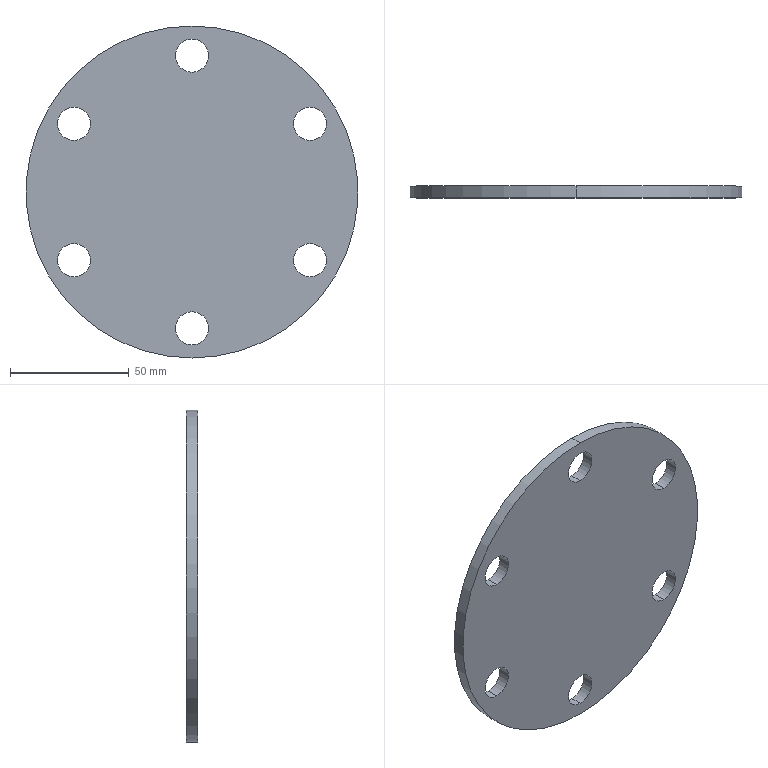Part | STEP file | OP10-030_plate | 1 solid | 16 faces | box 140 x 5 x 140 mm | volume 72351 mm3 | cylinder 14 | plane 2 | commonest cylinder face diameters 14 x12 140 x2
STEP:
#1=CARTESIAN_POINT('',(0.,0.,0.));
#2=DIRECTION('',(0.,0.,1.));
#3=DIRECTION('',(1.,0.,0.));
#4=AXIS2_PLACEMENT_3D('',#1,#2,#3);
#5=CARTESIAN_POINT('',(-49.796,0.,-21.75));
#6=VERTEX_POINT('',#5);
#7=CARTESIAN_POINT('',(-49.796,5.,-21.75));
#8=VERTEX_POINT('',#7);
#9=CARTESIAN_POINT('',(-49.796,0.,-21.75));
#10=DIRECTION('',(0.,1.,0.));
#11=VECTOR('',#10,1.);
#12=LINE('',#9,#11);
#13=CARTESIAN_POINT('',(-49.796,0.,-28.75));
#14=DIRECTION('',(0.,1.,0.));
#15=DIRECTION('',(0.,0.,1.));
#16=AXIS2_PLACEMENT_3D('',#13,#14,#15);
#17=CYLINDRICAL_SURFACE('',#16,7.);
#18=CARTESIAN_POINT('',(6.283,0.));
#19=DIRECTION('',(0.,1.));
#20=VECTOR('',#19,1.);
#21=LINE('',#18,#20);
#22=(GEOMETRIC_REPRESENTATION_CONTEXT(2)PARAMETRIC_REPRESENTATION_CONTEXT()REPRESENTATION_CONTEXT('',''));
#23=DEFINITIONAL_REPRESENTATION('',(#21),#22);
#24=PCURVE('',#17,#23);
#25=CARTESIAN_POINT('',(-49.796,0.,-28.75));
#26=DIRECTION('',(0.,1.,0.));
#27=DIRECTION('',(0.,0.,1.));
#28=AXIS2_PLACEMENT_3D('',#25,#26,#27);
#29=CYLINDRICAL_SURFACE('',#28,7.);
#30=CARTESIAN_POINT('',(0.,0.));
#31=DIRECTION('',(0.,1.));
#32=VECTOR('',#31,1.);
#33=LINE('',#30,#32);
#34=(GEOMETRIC_REPRESENTATION_CONTEXT(2)PARAMETRIC_REPRESENTATION_CONTEXT()REPRESENTATION_CONTEXT('',''));
#35=DEFINITIONAL_REPRESENTATION('',(#33),#34);
#36=PCURVE('',#29,#35);
#37=SURFACE_CURVE('',#12,(#24,#36),.PCURVE_S1.);
#38=EDGE_CURVE('',#6,#8,#37,.T.);
#39=ORIENTED_EDGE('',*,*,#38,.T.);
#40=CARTESIAN_POINT('',(-49.796,5.,-35.75));
#41=VERTEX_POINT('',#40);
#42=CARTESIAN_POINT('',(-49.796,5.,-28.75));
#43=DIRECTION('',(0.,1.,0.));
#44=DIRECTION('',(0.866,0.,0.5));
#45=AXIS2_PLACEMENT_3D('',#42,#43,#44);
#46=CIRCLE('',#45,7.);
#47=CARTESIAN_POINT('',(1.047,5.));
#48=DIRECTION('',(1.,0.));
#49=VECTOR('',#48,1.);
#50=LINE('',#47,#49);
#51=(GEOMETRIC_REPRESENTATION_CONTEXT(2)PARAMETRIC_REPRESENTATION_CONTEXT()REPRESENTATION_CONTEXT('',''));
#52=DEFINITIONAL_REPRESENTATION('',(#50),#51);
#53=PCURVE('',#17,#52);
#54=CARTESIAN_POINT('',(0.,5.,0.));
#55=DIRECTION('',(0.,1.,0.));
#56=DIRECTION('',(0.,0.,1.));
#57=AXIS2_PLACEMENT_3D('',#54,#55,#56);
#58=PLANE('',#57);
#59=CARTESIAN_POINT('',(-28.75,-49.796));
#60=DIRECTION('',(0.5,0.866));
#61=AXIS2_PLACEMENT_2D('',#59,#60);
#62=CIRCLE('',#61,7.);
#63=(GEOMETRIC_REPRESENTATION_CONTEXT(2)PARAMETRIC_REPRESENTATION_CONTEXT()REPRESENTATION_CONTEXT('',''));
#64=DEFINITIONAL_REPRESENTATION('',(#62),#63);
#65=PCURVE('',#58,#64);
#66=SURFACE_CURVE('',#46,(#53,#65),.PCURVE_S1.);
#67=EDGE_CURVE('',#41,#8,#66,.T.);
#68=ORIENTED_EDGE('',*,*,#67,.F.);
#69=CARTESIAN_POINT('',(-49.796,0.,-35.75));
#70=VERTEX_POINT('',#69);
#71=CARTESIAN_POINT('',(-49.796,0.,-35.75));
#72=DIRECTION('',(0.,1.,0.));
#73=VECTOR('',#72,1.);
#74=LINE('',#71,#73);
#75=CARTESIAN_POINT('',(3.142,0.));
#76=DIRECTION('',(0.,1.));
#77=VECTOR('',#76,1.);
#78=LINE('',#75,#77);
#79=(GEOMETRIC_REPRESENTATION_CONTEXT(2)PARAMETRIC_REPRESENTATION_CONTEXT()REPRESENTATION_CONTEXT('',''));
#80=DEFINITIONAL_REPRESENTATION('',(#78),#79);
#81=PCURVE('',#17,#80);
#82=CARTESIAN_POINT('',(3.142,0.));
#83=DIRECTION('',(0.,1.));
#84=VECTOR('',#83,1.);
#85=LINE('',#82,#84);
#86=(GEOMETRIC_REPRESENTATION_CONTEXT(2)PARAMETRIC_REPRESENTATION_CONTEXT()REPRESENTATION_CONTEXT('',''));
#87=DEFINITIONAL_REPRESENTATION('',(#85),#86);
#88=PCURVE('',#29,#87);
#89=SURFACE_CURVE('',#74,(#81,#88),.PCURVE_S1.);
#90=EDGE_CURVE('',#70,#41,#89,.T.);
#91=ORIENTED_EDGE('',*,*,#90,.F.);
#92=CARTESIAN_POINT('',(-49.796,0.,-28.75));
#93=DIRECTION('',(0.,1.,0.));
#94=DIRECTION('',(0.866,0.,0.5));
#95=AXIS2_PLACEMENT_3D('',#92,#93,#94);
#96=CIRCLE('',#95,7.);
#97=CARTESIAN_POINT('',(1.047,0.));
#98=DIRECTION('',(1.,0.));
#99=VECTOR('',#98,1.);
#100=LINE('',#97,#99);
#101=(GEOMETRIC_REPRESENTATION_CONTEXT(2)PARAMETRIC_REPRESENTATION_CONTEXT()REPRESENTATION_CONTEXT('',''));
#102=DEFINITIONAL_REPRESENTATION('',(#100),#101);
#103=PCURVE('',#17,#102);
#104=CARTESIAN_POINT('',(0.,0.,0.));
#105=DIRECTION('',(0.,1.,0.));
#106=DIRECTION('',(0.,0.,1.));
#107=AXIS2_PLACEMENT_3D('',#104,#105,#106);
#108=PLANE('',#107);
#109=CARTESIAN_POINT('',(-28.75,-49.796));
#110=DIRECTION('',(0.5,0.866));
#111=AXIS2_PLACEMENT_2D('',#109,#110);
#112=CIRCLE('',#111,7.);
#113=(GEOMETRIC_REPRESENTATION_CONTEXT(2)PARAMETRIC_REPRESENTATION_CONTEXT()REPRESENTATION_CONTEXT('',''));
#114=DEFINITIONAL_REPRESENTATION('',(#112),#113);
#115=PCURVE('',#108,#114);
#116=SURFACE_CURVE('',#96,(#103,#115),.PCURVE_S1.);
#117=EDGE_CURVE('',#70,#6,#116,.T.);
#118=ORIENTED_EDGE('',*,*,#117,.T.);
#119=EDGE_LOOP('',(#39,#68,#91,#118));
#120=FACE_BOUND('',#119,.F.);
#121=ADVANCED_FACE('',(#120),#17,.F.);
#122=CARTESIAN_POINT('',(-49.796,0.,35.75));
#123=VERTEX_POINT('',#122);
#124=CARTESIAN_POINT('',(-49.796,5.,35.75));
#125=VERTEX_POINT('',#124);
#126=CARTESIAN_POINT('',(-49.796,0.,35.75));
#127=DIRECTION('',(0.,1.,0.));
#128=VECTOR('',#127,1.);
#129=LINE('',#126,#128);
#130=CARTESIAN_POINT('',(-49.796,0.,28.75));
#131=DIRECTION('',(0.,1.,0.));
#132=DIRECTION('',(0.,0.,1.));
#133=AXIS2_PLACEMENT_3D('',#130,#131,#132);
#134=CYLINDRICAL_SURFACE('',#133,7.);
#135=CARTESIAN_POINT('',(6.283,0.));
#136=DIRECTION('',(0.,1.));
#137=VECTOR('',#136,1.);
#138=LINE('',#135,#137);
#139=(GEOMETRIC_REPRESENTATION_CONTEXT(2)PARAMETRIC_REPRESENTATION_CONTEXT()REPRESENTATION_CONTEXT('',''));
#140=DEFINITIONAL_REPRESENTATION('',(#138),#139);
#141=PCURVE('',#134,#140);
#142=CARTESIAN_POINT('',(-49.796,0.,28.75));
#143=DIRECTION('',(0.,1.,0.));
#144=DIRECTION('',(0.,0.,1.));
#145=AXIS2_PLACEMENT_3D('',#142,#143,#144);
#146=CYLINDRICAL_SURFACE('',#145,7.);
#147=CARTESIAN_POINT('',(0.,0.));
#148=DIRECTION('',(0.,1.));
#149=VECTOR('',#148,1.);
#150=LINE('',#147,#149);
#151=(GEOMETRIC_REPRESENTATION_CONTEXT(2)PARAMETRIC_REPRESENTATION_CONTEXT()REPRESENTATION_CONTEXT('',''));
#152=DEFINITIONAL_REPRESENTATION('',(#150),#151);
#153=PCURVE('',#146,#152);
#154=SURFACE_CURVE('',#129,(#141,#153),.PCURVE_S1.);
#155=EDGE_CURVE('',#123,#125,#154,.T.);
#156=ORIENTED_EDGE('',*,*,#155,.T.);
#157=CARTESIAN_POINT('',(-49.796,5.,21.75));
#158=VERTEX_POINT('',#157);
#159=CARTESIAN_POINT('',(-49.796,5.,28.75));
#160=DIRECTION('',(0.,1.,0.));
#161=DIRECTION('',(0.866,0.,-0.5));
#162=AXIS2_PLACEMENT_3D('',#159,#160,#161);
#163=CIRCLE('',#162,7.);
#164=CARTESIAN_POINT('',(2.094,5.));
#165=DIRECTION('',(1.,0.));
#166=VECTOR('',#165,1.);
#167=LINE('',#164,#166);
#168=(GEOMETRIC_REPRESENTATION_CONTEXT(2)PARAMETRIC_REPRESENTATION_CONTEXT()REPRESENTATION_CONTEXT('',''));
#169=DEFINITIONAL_REPRESENTATION('',(#167),#168);
#170=PCURVE('',#134,#169);
#171=CARTESIAN_POINT('',(28.75,-49.796));
#172=DIRECTION('',(-0.5,0.866));
#173=AXIS2_PLACEMENT_2D('',#171,#172);
#174=CIRCLE('',#173,7.);
#175=(GEOMETRIC_REPRESENTATION_CONTEXT(2)PARAMETRIC_REPRESENTATION_CONTEXT()REPRESENTATION_CONTEXT('',''));
#176=DEFINITIONAL_REPRESENTATION('',(#174),#175);
#177=PCURVE('',#58,#176);
#178=SURFACE_CURVE('',#163,(#170,#177),.PCURVE_S1.);
#179=EDGE_CURVE('',#158,#125,#178,.T.);
#180=ORIENTED_EDGE('',*,*,#179,.F.);
#181=CARTESIAN_POINT('',(-49.796,0.,21.75));
#182=VERTEX_POINT('',#181);
#183=CARTESIAN_POINT('',(-49.796,0.,21.75));
#184=DIRECTION('',(0.,1.,0.));
#185=VECTOR('',#184,1.);
#186=LINE('',#183,#185);
#187=CARTESIAN_POINT('',(3.142,0.));
#188=DIRECTION('',(0.,1.));
#189=VECTOR('',#188,1.);
#190=LINE('',#187,#189);
#191=(GEOMETRIC_REPRESENTATION_CONTEXT(2)PARAMETRIC_REPRESENTATION_CONTEXT()REPRESENTATION_CONTEXT('',''));
#192=DEFINITIONAL_REPRESENTATION('',(#190),#191);
#193=PCURVE('',#134,#192);
#194=CARTESIAN_POINT('',(3.142,0.));
#195=DIRECTION('',(0.,1.));
#196=VECTOR('',#195,1.);
#197=LINE('',#194,#196);
#198=(GEOMETRIC_REPRESENTATION_CONTEXT(2)PARAMETRIC_REPRESENTATION_CONTEXT()REPRESENTATION_CONTEXT('',''));
#199=DEFINITIONAL_REPRESENTATION('',(#197),#198);
#200=PCURVE('',#146,#199);
#201=SURFACE_CURVE('',#186,(#193,#200),.PCURVE_S1.);
#202=EDGE_CURVE('',#182,#158,#201,.T.);
#203=ORIENTED_EDGE('',*,*,#202,.F.);
#204=CARTESIAN_POINT('',(-49.796,0.,28.75));
#205=DIRECTION('',(0.,1.,0.));
#206=DIRECTION('',(0.866,0.,-0.5));
#207=AXIS2_PLACEMENT_3D('',#204,#205,#206);
#208=CIRCLE('',#207,7.);
#209=CARTESIAN_POINT('',(2.094,0.));
#210=DIRECTION('',(1.,0.));
#211=VECTOR('',#210,1.);
#212=LINE('',#209,#211);
#213=(GEOMETRIC_REPRESENTATION_CONTEXT(2)PARAMETRIC_REPRESENTATION_CONTEXT()REPRESENTATION_CONTEXT('',''));
#214=DEFINITIONAL_REPRESENTATION('',(#212),#213);
#215=PCURVE('',#134,#214);
#216=CARTESIAN_POINT('',(28.75,-49.796));
#217=DIRECTION('',(-0.5,0.866));
#218=AXIS2_PLACEMENT_2D('',#216,#217);
#219=CIRCLE('',#218,7.);
#220=(GEOMETRIC_REPRESENTATION_CONTEXT(2)PARAMETRIC_REPRESENTATION_CONTEXT()REPRESENTATION_CONTEXT('',''));
#221=DEFINITIONAL_REPRESENTATION('',(#219),#220);
#222=PCURVE('',#108,#221);
#223=SURFACE_CURVE('',#208,(#215,#222),.PCURVE_S1.);
#224=EDGE_CURVE('',#182,#123,#223,.T.);
#225=ORIENTED_EDGE('',*,*,#224,.T.);
#226=EDGE_LOOP('',(#156,#180,#203,#225));
#227=FACE_BOUND('',#226,.F.);
#228=ADVANCED_FACE('',(#227),#134,.F.);
#229=CARTESIAN_POINT('',(0.,0.,64.5));
#230=VERTEX_POINT('',#229);
#231=CARTESIAN_POINT('',(0.,5.,64.5));
#232=VERTEX_POINT('',#231);
#233=CARTESIAN_POINT('',(0.,0.,64.5));
#234=DIRECTION('',(0.,1.,0.));
#235=VECTOR('',#234,1.);
#236=LINE('',#233,#235);
#237=CARTESIAN_POINT('',(0.,0.,57.5));
#238=DIRECTION('',(0.,1.,0.));
#239=DIRECTION('',(0.,0.,1.));
#240=AXIS2_PLACEMENT_3D('',#237,#238,#239);
#241=CYLINDRICAL_SURFACE('',#240,7.);
#242=CARTESIAN_POINT('',(6.283,0.));
#243=DIRECTION('',(0.,1.));
#244=VECTOR('',#243,1.);
#245=LINE('',#242,#244);
#246=(GEOMETRIC_REPRESENTATION_CONTEXT(2)PARAMETRIC_REPRESENTATION_CONTEXT()REPRESENTATION_CONTEXT('',''));
#247=DEFINITIONAL_REPRESENTATION('',(#245),#246);
#248=PCURVE('',#241,#247);
#249=CARTESIAN_POINT('',(0.,0.,57.5));
#250=DIRECTION('',(0.,1.,0.));
#251=DIRECTION('',(0.,0.,1.));
#252=AXIS2_PLACEMENT_3D('',#249,#250,#251);
#253=CYLINDRICAL_SURFACE('',#252,7.);
#254=CARTESIAN_POINT('',(0.,0.));
#255=DIRECTION('',(0.,1.));
#256=VECTOR('',#255,1.);
#257=LINE('',#254,#256);
#258=(GEOMETRIC_REPRESENTATION_CONTEXT(2)PARAMETRIC_REPRESENTATION_CONTEXT()REPRESENTATION_CONTEXT('',''));
#259=DEFINITIONAL_REPRESENTATION('',(#257),#258);
#260=PCURVE('',#253,#259);
#261=SURFACE_CURVE('',#236,(#248,#260),.PCURVE_S1.);
#262=EDGE_CURVE('',#230,#232,#261,.T.);
#263=ORIENTED_EDGE('',*,*,#262,.T.);
#264=CARTESIAN_POINT('',(0.,5.,50.5));
#265=VERTEX_POINT('',#264);
#266=CARTESIAN_POINT('',(0.,5.,57.5));
#267=DIRECTION('',(0.,1.,0.));
#268=DIRECTION('',(0.,0.,-1.));
#269=AXIS2_PLACEMENT_3D('',#266,#267,#268);
#270=CIRCLE('',#269,7.);
#271=CARTESIAN_POINT('',(3.142,5.));
#272=DIRECTION('',(1.,0.));
#273=VECTOR('',#272,1.);
#274=LINE('',#271,#273);
#275=(GEOMETRIC_REPRESENTATION_CONTEXT(2)PARAMETRIC_REPRESENTATION_CONTEXT()REPRESENTATION_CONTEXT('',''));
#276=DEFINITIONAL_REPRESENTATION('',(#274),#275);
#277=PCURVE('',#241,#276);
#278=CARTESIAN_POINT('',(57.5,0.));
#279=DIRECTION('',(-1.,0.));
#280=AXIS2_PLACEMENT_2D('',#278,#279);
#281=CIRCLE('',#280,7.);
#282=(GEOMETRIC_REPRESENTATION_CONTEXT(2)PARAMETRIC_REPRESENTATION_CONTEXT()REPRESENTATION_CONTEXT('',''));
#283=DEFINITIONAL_REPRESENTATION('',(#281),#282);
#284=PCURVE('',#58,#283);
#285=SURFACE_CURVE('',#270,(#277,#284),.PCURVE_S1.);
#286=EDGE_CURVE('',#265,#232,#285,.T.);
#287=ORIENTED_EDGE('',*,*,#286,.F.);
#288=CARTESIAN_POINT('',(0.,0.,50.5));
#289=VERTEX_POINT('',#288);
#290=CARTESIAN_POINT('',(0.,0.,50.5));
#291=DIRECTION('',(0.,1.,0.));
#292=VECTOR('',#291,1.);
#293=LINE('',#290,#292);
#294=CARTESIAN_POINT('',(3.142,0.));
#295=DIRECTION('',(0.,1.));
#296=VECTOR('',#295,1.);
#297=LINE('',#294,#296);
#298=(GEOMETRIC_REPRESENTATION_CONTEXT(2)PARAMETRIC_REPRESENTATION_CONTEXT()REPRESENTATION_CONTEXT('',''));
#299=DEFINITIONAL_REPRESENTATION('',(#297),#298);
#300=PCURVE('',#241,#299);
#301=CARTESIAN_POINT('',(3.142,0.));
#302=DIRECTION('',(0.,1.));
#303=VECTOR('',#302,1.);
#304=LINE('',#301,#303);
#305=(GEOMETRIC_REPRESENTATION_CONTEXT(2)PARAMETRIC_REPRESENTATION_CONTEXT()REPRESENTATION_CONTEXT('',''));
#306=DEFINITIONAL_REPRESENTATION('',(#304),#305);
#307=PCURVE('',#253,#306);
#308=SURFACE_CURVE('',#293,(#300,#307),.PCURVE_S1.);
#309=EDGE_CURVE('',#289,#265,#308,.T.);
#310=ORIENTED_EDGE('',*,*,#309,.F.);
#311=CARTESIAN_POINT('',(0.,0.,57.5));
#312=DIRECTION('',(0.,1.,0.));
#313=DIRECTION('',(0.,0.,-1.));
#314=AXIS2_PLACEMENT_3D('',#311,#312,#313);
#315=CIRCLE('',#314,7.);
#316=CARTESIAN_POINT('',(3.142,0.));
#317=DIRECTION('',(1.,0.));
#318=VECTOR('',#317,1.);
#319=LINE('',#316,#318);
#320=(GEOMETRIC_REPRESENTATION_CONTEXT(2)PARAMETRIC_REPRESENTATION_CONTEXT()REPRESENTATION_CONTEXT('',''));
#321=DEFINITIONAL_REPRESENTATION('',(#319),#320);
#322=PCURVE('',#241,#321);
#323=CARTESIAN_POINT('',(57.5,0.));
#324=DIRECTION('',(-1.,0.));
#325=AXIS2_PLACEMENT_2D('',#323,#324);
#326=CIRCLE('',#325,7.);
#327=(GEOMETRIC_REPRESENTATION_CONTEXT(2)PARAMETRIC_REPRESENTATION_CONTEXT()REPRESENTATION_CONTEXT('',''));
#328=DEFINITIONAL_REPRESENTATION('',(#326),#327);
#329=PCURVE('',#108,#328);
#330=SURFACE_CURVE('',#315,(#322,#329),.PCURVE_S1.);
#331=EDGE_CURVE('',#289,#230,#330,.T.);
#332=ORIENTED_EDGE('',*,*,#331,.T.);
#333=EDGE_LOOP('',(#263,#287,#310,#332));
#334=FACE_BOUND('',#333,.F.);
#335=ADVANCED_FACE('',(#334),#241,.F.);
#336=CARTESIAN_POINT('',(49.796,0.,35.75));
#337=VERTEX_POINT('',#336);
#338=CARTESIAN_POINT('',(49.796,5.,35.75));
#339=VERTEX_POINT('',#338);
#340=CARTESIAN_POINT('',(49.796,0.,35.75));
#341=DIRECTION('',(0.,1.,0.));
#342=VECTOR('',#341,1.);
#343=LINE('',#340,#342);
#344=CARTESIAN_POINT('',(49.796,0.,28.75));
#345=DIRECTION('',(0.,1.,0.));
#346=DIRECTION('',(0.,0.,1.));
#347=AXIS2_PLACEMENT_3D('',#344,#345,#346);
#348=CYLINDRICAL_SURFACE('',#347,7.);
#349=CARTESIAN_POINT('',(6.283,0.));
#350=DIRECTION('',(0.,1.));
#351=VECTOR('',#350,1.);
#352=LINE('',#349,#351);
#353=(GEOMETRIC_REPRESENTATION_CONTEXT(2)PARAMETRIC_REPRESENTATION_CONTEXT()REPRESENTATION_CONTEXT('',''));
#354=DEFINITIONAL_REPRESENTATION('',(#352),#353);
#355=PCURVE('',#348,#354);
#356=CARTESIAN_POINT('',(49.796,0.,28.75));
#357=DIRECTION('',(0.,1.,0.));
#358=DIRECTION('',(0.,0.,1.));
#359=AXIS2_PLACEMENT_3D('',#356,#357,#358);
#360=CYLINDRICAL_SURFACE('',#359,7.);
#361=CARTESIAN_POINT('',(0.,0.));
#362=DIRECTION('',(0.,1.));
#363=VECTOR('',#362,1.);
#364=LINE('',#361,#363);
#365=(GEOMETRIC_REPRESENTATION_CONTEXT(2)PARAMETRIC_REPRESENTATION_CONTEXT()REPRESENTATION_CONTEXT('',''));
#366=DEFINITIONAL_REPRESENTATION('',(#364),#365);
#367=PCURVE('',#360,#366);
#368=SURFACE_CURVE('',#343,(#355,#367),.PCURVE_S1.);
#369=EDGE_CURVE('',#337,#339,#368,.T.);
#370=ORIENTED_EDGE('',*,*,#369,.T.);
#371=CARTESIAN_POINT('',(49.796,5.,21.75));
#372=VERTEX_POINT('',#371);
#373=CARTESIAN_POINT('',(49.796,5.,28.75));
#374=DIRECTION('',(0.,1.,0.));
#375=DIRECTION('',(-0.866,0.,-0.5));
#376=AXIS2_PLACEMENT_3D('',#373,#374,#375);
#377=CIRCLE('',#376,7.);
#378=CARTESIAN_POINT('',(-2.094,5.));
#379=DIRECTION('',(1.,0.));
#380=VECTOR('',#379,1.);
#381=LINE('',#378,#380);
#382=(GEOMETRIC_REPRESENTATION_CONTEXT(2)PARAMETRIC_REPRESENTATION_CONTEXT()REPRESENTATION_CONTEXT('',''));
#383=DEFINITIONAL_REPRESENTATION('',(#381),#382);
#384=PCURVE('',#348,#383);
#385=CARTESIAN_POINT('',(28.75,49.796));
#386=DIRECTION('',(-0.5,-0.866));
#387=AXIS2_PLACEMENT_2D('',#385,#386);
#388=CIRCLE('',#387,7.);
#389=(GEOMETRIC_REPRESENTATION_CONTEXT(2)PARAMETRIC_REPRESENTATION_CONTEXT()REPRESENTATION_CONTEXT('',''));
#390=DEFINITIONAL_REPRESENTATION('',(#388),#389);
#391=PCURVE('',#58,#390);
#392=SURFACE_CURVE('',#377,(#384,#391),.PCURVE_S1.);
#393=EDGE_CURVE('',#372,#339,#392,.T.);
#394=ORIENTED_EDGE('',*,*,#393,.F.);
#395=CARTESIAN_POINT('',(49.796,0.,21.75));
#396=VERTEX_POINT('',#395);
#397=CARTESIAN_POINT('',(49.796,0.,21.75));
#398=DIRECTION('',(0.,1.,0.));
#399=VECTOR('',#398,1.);
#400=LINE('',#397,#399);
#401=CARTESIAN_POINT('',(3.142,0.));
#402=DIRECTION('',(0.,1.));
#403=VECTOR('',#402,1.);
#404=LINE('',#401,#403);
#405=(GEOMETRIC_REPRESENTATION_CONTEXT(2)PARAMETRIC_REPRESENTATION_CONTEXT()REPRESENTATION_CONTEXT('',''));
#406=DEFINITIONAL_REPRESENTATION('',(#404),#405);
#407=PCURVE('',#348,#406);
#408=CARTESIAN_POINT('',(3.142,0.));
#409=DIRECTION('',(0.,1.));
#410=VECTOR('',#409,1.);
#411=LINE('',#408,#410);
#412=(GEOMETRIC_REPRESENTATION_CONTEXT(2)PARAMETRIC_REPRESENTATION_CONTEXT()REPRESENTATION_CONTEXT('',''));
#413=DEFINITIONAL_REPRESENTATION('',(#411),#412);
#414=PCURVE('',#360,#413);
#415=SURFACE_CURVE('',#400,(#407,#414),.PCURVE_S1.);
#416=EDGE_CURVE('',#396,#372,#415,.T.);
#417=ORIENTED_EDGE('',*,*,#416,.F.);
#418=CARTESIAN_POINT('',(49.796,0.,28.75));
#419=DIRECTION('',(0.,1.,0.));
#420=DIRECTION('',(-0.866,0.,-0.5));
#421=AXIS2_PLACEMENT_3D('',#418,#419,#420);
#422=CIRCLE('',#421,7.);
#423=CARTESIAN_POINT('',(-2.094,0.));
#424=DIRECTION('',(1.,0.));
#425=VECTOR('',#424,1.);
#426=LINE('',#423,#425);
#427=(GEOMETRIC_REPRESENTATION_CONTEXT(2)PARAMETRIC_REPRESENTATION_CONTEXT()REPRESENTATION_CONTEXT('',''));
#428=DEFINITIONAL_REPRESENTATION('',(#426),#427);
#429=PCURVE('',#348,#428);
#430=CARTESIAN_POINT('',(28.75,49.796));
#431=DIRECTION('',(-0.5,-0.866));
#432=AXIS2_PLACEMENT_2D('',#430,#431);
#433=CIRCLE('',#432,7.);
#434=(GEOMETRIC_REPRESENTATION_CONTEXT(2)PARAMETRIC_REPRESENTATION_CONTEXT()REPRESENTATION_CONTEXT('',''));
#435=DEFINITIONAL_REPRESENTATION('',(#433),#434);
#436=PCURVE('',#108,#435);
#437=SURFACE_CURVE('',#422,(#429,#436),.PCURVE_S1.);
#438=EDGE_CURVE('',#396,#337,#437,.T.);
#439=ORIENTED_EDGE('',*,*,#438,.T.);
#440=EDGE_LOOP('',(#370,#394,#417,#439));
#441=FACE_BOUND('',#440,.F.);
#442=ADVANCED_FACE('',(#441),#348,.F.);
#443=CARTESIAN_POINT('',(49.796,0.,-21.75));
#444=VERTEX_POINT('',#443);
#445=CARTESIAN_POINT('',(49.796,5.,-21.75));
#446=VERTEX_POINT('',#445);
#447=CARTESIAN_POINT('',(49.796,0.,-21.75));
#448=DIRECTION('',(0.,1.,0.));
#449=VECTOR('',#448,1.);
#450=LINE('',#447,#449);
#451=CARTESIAN_POINT('',(49.796,0.,-28.75));
#452=DIRECTION('',(0.,1.,0.));
#453=DIRECTION('',(0.,0.,1.));
#454=AXIS2_PLACEMENT_3D('',#451,#452,#453);
#455=CYLINDRICAL_SURFACE('',#454,7.);
#456=CARTESIAN_POINT('',(6.283,0.));
#457=DIRECTION('',(0.,1.));
#458=VECTOR('',#457,1.);
#459=LINE('',#456,#458);
#460=(GEOMETRIC_REPRESENTATION_CONTEXT(2)PARAMETRIC_REPRESENTATION_CONTEXT()REPRESENTATION_CONTEXT('',''));
#461=DEFINITIONAL_REPRESENTATION('',(#459),#460);
#462=PCURVE('',#455,#461);
#463=CARTESIAN_POINT('',(49.796,0.,-28.75));
#464=DIRECTION('',(0.,1.,0.));
#465=DIRECTION('',(0.,0.,1.));
#466=AXIS2_PLACEMENT_3D('',#463,#464,#465);
#467=CYLINDRICAL_SURFACE('',#466,7.);
#468=CARTESIAN_POINT('',(0.,0.));
#469=DIRECTION('',(0.,1.));
#470=VECTOR('',#469,1.);
#471=LINE('',#468,#470);
#472=(GEOMETRIC_REPRESENTATION_CONTEXT(2)PARAMETRIC_REPRESENTATION_CONTEXT()REPRESENTATION_CONTEXT('',''));
#473=DEFINITIONAL_REPRESENTATION('',(#471),#472);
#474=PCURVE('',#467,#473);
#475=SURFACE_CURVE('',#450,(#462,#474),.PCURVE_S1.);
#476=EDGE_CURVE('',#444,#446,#475,.T.);
#477=ORIENTED_EDGE('',*,*,#476,.T.);
#478=CARTESIAN_POINT('',(49.796,5.,-35.75));
#479=VERTEX_POINT('',#478);
#480=CARTESIAN_POINT('',(49.796,5.,-28.75));
#481=DIRECTION('',(0.,1.,0.));
#482=DIRECTION('',(-0.866,0.,0.5));
#483=AXIS2_PLACEMENT_3D('',#480,#481,#482);
#484=CIRCLE('',#483,7.);
#485=CARTESIAN_POINT('',(-1.047,5.));
#486=DIRECTION('',(1.,0.));
#487=VECTOR('',#486,1.);
#488=LINE('',#485,#487);
#489=(GEOMETRIC_REPRESENTATION_CONTEXT(2)PARAMETRIC_REPRESENTATION_CONTEXT()REPRESENTATION_CONTEXT('',''));
#490=DEFINITIONAL_REPRESENTATION('',(#488),#489);
#491=PCURVE('',#455,#490);
#492=CARTESIAN_POINT('',(-28.75,49.796));
#493=DIRECTION('',(0.5,-0.866));
#494=AXIS2_PLACEMENT_2D('',#492,#493);
#495=CIRCLE('',#494,7.);
#496=(GEOMETRIC_REPRESENTATION_CONTEXT(2)PARAMETRIC_REPRESENTATION_CONTEXT()REPRESENTATION_CONTEXT('',''));
#497=DEFINITIONAL_REPRESENTATION('',(#495),#496);
#498=PCURVE('',#58,#497);
#499=SURFACE_CURVE('',#484,(#491,#498),.PCURVE_S1.);
#500=EDGE_CURVE('',#479,#446,#499,.T.);
#501=ORIENTED_EDGE('',*,*,#500,.F.);
#502=CARTESIAN_POINT('',(49.796,0.,-35.75));
#503=VERTEX_POINT('',#502);
#504=CARTESIAN_POINT('',(49.796,0.,-35.75));
#505=DIRECTION('',(0.,1.,0.));
#506=VECTOR('',#505,1.);
#507=LINE('',#504,#506);
#508=CARTESIAN_POINT('',(3.142,0.));
#509=DIRECTION('',(0.,1.));
#510=VECTOR('',#509,1.);
#511=LINE('',#508,#510);
#512=(GEOMETRIC_REPRESENTATION_CONTEXT(2)PARAMETRIC_REPRESENTATION_CONTEXT()REPRESENTATION_CONTEXT('',''));
#513=DEFINITIONAL_REPRESENTATION('',(#511),#512);
#514=PCURVE('',#455,#513);
#515=CARTESIAN_POINT('',(3.142,0.));
#516=DIRECTION('',(0.,1.));
#517=VECTOR('',#516,1.);
#518=LINE('',#515,#517);
#519=(GEOMETRIC_REPRESENTATION_CONTEXT(2)PARAMETRIC_REPRESENTATION_CONTEXT()REPRESENTATION_CONTEXT('',''));
#520=DEFINITIONAL_REPRESENTATION('',(#518),#519);
#521=PCURVE('',#467,#520);
#522=SURFACE_CURVE('',#507,(#514,#521),.PCURVE_S1.);
#523=EDGE_CURVE('',#503,#479,#522,.T.);
#524=ORIENTED_EDGE('',*,*,#523,.F.);
#525=CARTESIAN_POINT('',(49.796,0.,-28.75));
#526=DIRECTION('',(0.,1.,0.));
#527=DIRECTION('',(-0.866,0.,0.5));
#528=AXIS2_PLACEMENT_3D('',#525,#526,#527);
#529=CIRCLE('',#528,7.);
#530=CARTESIAN_POINT('',(-1.047,0.));
#531=DIRECTION('',(1.,0.));
#532=VECTOR('',#531,1.);
#533=LINE('',#530,#532);
#534=(GEOMETRIC_REPRESENTATION_CONTEXT(2)PARAMETRIC_REPRESENTATION_CONTEXT()REPRESENTATION_CONTEXT('',''));
#535=DEFINITIONAL_REPRESENTATION('',(#533),#534);
#536=PCURVE('',#455,#535);
#537=CARTESIAN_POINT('',(-28.75,49.796));
#538=DIRECTION('',(0.5,-0.866));
#539=AXIS2_PLACEMENT_2D('',#537,#538);
#540=CIRCLE('',#539,7.);
#541=(GEOMETRIC_REPRESENTATION_CONTEXT(2)PARAMETRIC_REPRESENTATION_CONTEXT()REPRESENTATION_CONTEXT('',''));
#542=DEFINITIONAL_REPRESENTATION('',(#540),#541);
#543=PCURVE('',#108,#542);
#544=SURFACE_CURVE('',#529,(#536,#543),.PCURVE_S1.);
#545=EDGE_CURVE('',#503,#444,#544,.T.);
#546=ORIENTED_EDGE('',*,*,#545,.T.);
#547=EDGE_LOOP('',(#477,#501,#524,#546));
#548=FACE_BOUND('',#547,.F.);
#549=ADVANCED_FACE('',(#548),#455,.F.);
#550=CARTESIAN_POINT('',(0.,0.,-50.5));
#551=VERTEX_POINT('',#550);
#552=CARTESIAN_POINT('',(0.,5.,-50.5));
#553=VERTEX_POINT('',#552);
#554=CARTESIAN_POINT('',(0.,0.,-50.5));
#555=DIRECTION('',(0.,1.,0.));
#556=VECTOR('',#555,1.);
#557=LINE('',#554,#556);
#558=CARTESIAN_POINT('',(0.,0.,-57.5));
#559=DIRECTION('',(0.,1.,0.));
#560=DIRECTION('',(0.,0.,1.));
#561=AXIS2_PLACEMENT_3D('',#558,#559,#560);
#562=CYLINDRICAL_SURFACE('',#561,7.);
#563=CARTESIAN_POINT('',(6.283,0.));
#564=DIRECTION('',(0.,1.));
#565=VECTOR('',#564,1.);
#566=LINE('',#563,#565);
#567=(GEOMETRIC_REPRESENTATION_CONTEXT(2)PARAMETRIC_REPRESENTATION_CONTEXT()REPRESENTATION_CONTEXT('',''));
#568=DEFINITIONAL_REPRESENTATION('',(#566),#567);
#569=PCURVE('',#562,#568);
#570=CARTESIAN_POINT('',(0.,0.,-57.5));
#571=DIRECTION('',(0.,1.,0.));
#572=DIRECTION('',(0.,0.,1.));
#573=AXIS2_PLACEMENT_3D('',#570,#571,#572);
#574=CYLINDRICAL_SURFACE('',#573,7.);
#575=CARTESIAN_POINT('',(0.,0.));
#576=DIRECTION('',(0.,1.));
#577=VECTOR('',#576,1.);
#578=LINE('',#575,#577);
#579=(GEOMETRIC_REPRESENTATION_CONTEXT(2)PARAMETRIC_REPRESENTATION_CONTEXT()REPRESENTATION_CONTEXT('',''));
#580=DEFINITIONAL_REPRESENTATION('',(#578),#579);
#581=PCURVE('',#574,#580);
#582=SURFACE_CURVE('',#557,(#569,#581),.PCURVE_S1.);
#583=EDGE_CURVE('',#551,#553,#582,.T.);
#584=ORIENTED_EDGE('',*,*,#583,.T.);
#585=CARTESIAN_POINT('',(0.,5.,-64.5));
#586=VERTEX_POINT('',#585);
#587=CARTESIAN_POINT('',(0.,5.,-57.5));
#588=DIRECTION('',(0.,1.,0.));
#589=DIRECTION('',(0.,0.,1.));
#590=AXIS2_PLACEMENT_3D('',#587,#588,#589);
#591=CIRCLE('',#590,7.);
#592=CARTESIAN_POINT('',(0.,5.));
#593=DIRECTION('',(1.,0.));
#594=VECTOR('',#593,1.);
#595=LINE('',#592,#594);
#596=(GEOMETRIC_REPRESENTATION_CONTEXT(2)PARAMETRIC_REPRESENTATION_CONTEXT()REPRESENTATION_CONTEXT('',''));
#597=DEFINITIONAL_REPRESENTATION('',(#595),#596);
#598=PCURVE('',#562,#597);
#599=CARTESIAN_POINT('',(-57.5,0.));
#600=DIRECTION('',(1.,0.));
#601=AXIS2_PLACEMENT_2D('',#599,#600);
#602=CIRCLE('',#601,7.);
#603=(GEOMETRIC_REPRESENTATION_CONTEXT(2)PARAMETRIC_REPRESENTATION_CONTEXT()REPRESENTATION_CONTEXT('',''));
#604=DEFINITIONAL_REPRESENTATION('',(#602),#603);
#605=PCURVE('',#58,#604);
#606=SURFACE_CURVE('',#591,(#598,#605),.PCURVE_S1.);
#607=EDGE_CURVE('',#586,#553,#606,.T.);
#608=ORIENTED_EDGE('',*,*,#607,.F.);
#609=CARTESIAN_POINT('',(0.,0.,-64.5));
#610=VERTEX_POINT('',#609);
#611=CARTESIAN_POINT('',(0.,0.,-64.5));
#612=DIRECTION('',(0.,1.,0.));
#613=VECTOR('',#612,1.);
#614=LINE('',#611,#613);
#615=CARTESIAN_POINT('',(3.142,0.));
#616=DIRECTION('',(0.,1.));
#617=VECTOR('',#616,1.);
#618=LINE('',#615,#617);
#619=(GEOMETRIC_REPRESENTATION_CONTEXT(2)PARAMETRIC_REPRESENTATION_CONTEXT()REPRESENTATION_CONTEXT('',''));
#620=DEFINITIONAL_REPRESENTATION('',(#618),#619);
#621=PCURVE('',#562,#620);
#622=CARTESIAN_POINT('',(3.142,0.));
#623=DIRECTION('',(0.,1.));
#624=VECTOR('',#623,1.);
#625=LINE('',#622,#624);
#626=(GEOMETRIC_REPRESENTATION_CONTEXT(2)PARAMETRIC_REPRESENTATION_CONTEXT()REPRESENTATION_CONTEXT('',''));
#627=DEFINITIONAL_REPRESENTATION('',(#625),#626);
#628=PCURVE('',#574,#627);
#629=SURFACE_CURVE('',#614,(#621,#628),.PCURVE_S1.);
#630=EDGE_CURVE('',#610,#586,#629,.T.);
#631=ORIENTED_EDGE('',*,*,#630,.F.);
#632=CARTESIAN_POINT('',(0.,0.,-57.5));
#633=DIRECTION('',(0.,1.,0.));
#634=DIRECTION('',(0.,0.,1.));
#635=AXIS2_PLACEMENT_3D('',#632,#633,#634);
#636=CIRCLE('',#635,7.);
#637=CARTESIAN_POINT('',(0.,0.));
#638=DIRECTION('',(1.,0.));
#639=VECTOR('',#638,1.);
#640=LINE('',#637,#639);
#641=(GEOMETRIC_REPRESENTATION_CONTEXT(2)PARAMETRIC_REPRESENTATION_CONTEXT()REPRESENTATION_CONTEXT('',''));
#642=DEFINITIONAL_REPRESENTATION('',(#640),#641);
#643=PCURVE('',#562,#642);
#644=CARTESIAN_POINT('',(-57.5,0.));
#645=DIRECTION('',(1.,0.));
#646=AXIS2_PLACEMENT_2D('',#644,#645);
#647=CIRCLE('',#646,7.);
#648=(GEOMETRIC_REPRESENTATION_CONTEXT(2)PARAMETRIC_REPRESENTATION_CONTEXT()REPRESENTATION_CONTEXT('',''));
#649=DEFINITIONAL_REPRESENTATION('',(#647),#648);
#650=PCURVE('',#108,#649);
#651=SURFACE_CURVE('',#636,(#643,#650),.PCURVE_S1.);
#652=EDGE_CURVE('',#610,#551,#651,.T.);
#653=ORIENTED_EDGE('',*,*,#652,.T.);
#654=EDGE_LOOP('',(#584,#608,#631,#653));
#655=FACE_BOUND('',#654,.F.);
#656=ADVANCED_FACE('',(#655),#562,.F.);
#657=CARTESIAN_POINT('',(0.,5.,70.));
#658=VERTEX_POINT('',#657);
#659=CARTESIAN_POINT('',(0.,5.,-70.));
#660=VERTEX_POINT('',#659);
#661=CARTESIAN_POINT('',(0.,5.,0.));
#662=DIRECTION('',(0.,1.,0.));
#663=DIRECTION('',(0.,0.,1.));
#664=AXIS2_PLACEMENT_3D('',#661,#662,#663);
#665=CIRCLE('',#664,70.);
#666=CARTESIAN_POINT('',(0.,5.,0.));
#667=DIRECTION('',(0.,-1.,0.));
#668=DIRECTION('',(0.,0.,-1.));
#669=AXIS2_PLACEMENT_3D('',#666,#667,#668);
#670=CYLINDRICAL_SURFACE('',#669,70.);
#671=CARTESIAN_POINT('',(3.142,0.));
#672=DIRECTION('',(-1.,0.));
#673=VECTOR('',#672,1.);
#674=LINE('',#671,#673);
#675=(GEOMETRIC_REPRESENTATION_CONTEXT(2)PARAMETRIC_REPRESENTATION_CONTEXT()REPRESENTATION_CONTEXT('',''));
#676=DEFINITIONAL_REPRESENTATION('',(#674),#675);
#677=PCURVE('',#670,#676);
#678=CARTESIAN_POINT('',(0.,0.));
#679=DIRECTION('',(1.,0.));
#680=AXIS2_PLACEMENT_2D('',#678,#679);
#681=CIRCLE('',#680,70.);
#682=(GEOMETRIC_REPRESENTATION_CONTEXT(2)PARAMETRIC_REPRESENTATION_CONTEXT()REPRESENTATION_CONTEXT('',''));
#683=DEFINITIONAL_REPRESENTATION('',(#681),#682);
#684=PCURVE('',#58,#683);
#685=SURFACE_CURVE('',#665,(#677,#684),.PCURVE_S1.);
#686=EDGE_CURVE('',#658,#660,#685,.T.);
#687=ORIENTED_EDGE('',*,*,#686,.F.);
#688=CARTESIAN_POINT('',(0.,0.,70.));
#689=VERTEX_POINT('',#688);
#690=CARTESIAN_POINT('',(0.,5.,70.));
#691=DIRECTION('',(0.,-1.,0.));
#692=VECTOR('',#691,1.);
#693=LINE('',#690,#692);
#694=CARTESIAN_POINT('',(3.142,0.));
#695=DIRECTION('',(0.,1.));
#696=VECTOR('',#695,1.);
#697=LINE('',#694,#696);
#698=(GEOMETRIC_REPRESENTATION_CONTEXT(2)PARAMETRIC_REPRESENTATION_CONTEXT()REPRESENTATION_CONTEXT('',''));
#699=DEFINITIONAL_REPRESENTATION('',(#697),#698);
#700=PCURVE('',#670,#699);
#701=CARTESIAN_POINT('',(0.,5.,0.));
#702=DIRECTION('',(0.,-1.,0.));
#703=DIRECTION('',(0.,0.,-1.));
#704=AXIS2_PLACEMENT_3D('',#701,#702,#703);
#705=CYLINDRICAL_SURFACE('',#704,70.);
#706=CARTESIAN_POINT('',(3.142,0.));
#707=DIRECTION('',(0.,1.));
#708=VECTOR('',#707,1.);
#709=LINE('',#706,#708);
#710=(GEOMETRIC_REPRESENTATION_CONTEXT(2)PARAMETRIC_REPRESENTATION_CONTEXT()REPRESENTATION_CONTEXT('',''));
#711=DEFINITIONAL_REPRESENTATION('',(#709),#710);
#712=PCURVE('',#705,#711);
#713=SURFACE_CURVE('',#693,(#700,#712),.PCURVE_S1.);
#714=EDGE_CURVE('',#658,#689,#713,.T.);
#715=ORIENTED_EDGE('',*,*,#714,.T.);
#716=CARTESIAN_POINT('',(0.,0.,-70.));
#717=VERTEX_POINT('',#716);
#718=CARTESIAN_POINT('',(0.,0.,0.));
#719=DIRECTION('',(0.,1.,0.));
#720=DIRECTION('',(0.,0.,1.));
#721=AXIS2_PLACEMENT_3D('',#718,#719,#720);
#722=CIRCLE('',#721,70.);
#723=CARTESIAN_POINT('',(3.142,5.));
#724=DIRECTION('',(-1.,0.));
#725=VECTOR('',#724,1.);
#726=LINE('',#723,#725);
#727=(GEOMETRIC_REPRESENTATION_CONTEXT(2)PARAMETRIC_REPRESENTATION_CONTEXT()REPRESENTATION_CONTEXT('',''));
#728=DEFINITIONAL_REPRESENTATION('',(#726),#727);
#729=PCURVE('',#670,#728);
#730=CARTESIAN_POINT('',(0.,0.));
#731=DIRECTION('',(1.,0.));
#732=AXIS2_PLACEMENT_2D('',#730,#731);
#733=CIRCLE('',#732,70.);
#734=(GEOMETRIC_REPRESENTATION_CONTEXT(2)PARAMETRIC_REPRESENTATION_CONTEXT()REPRESENTATION_CONTEXT('',''));
#735=DEFINITIONAL_REPRESENTATION('',(#733),#734);
#736=PCURVE('',#108,#735);
#737=SURFACE_CURVE('',#722,(#729,#736),.PCURVE_S1.);
#738=EDGE_CURVE('',#689,#717,#737,.T.);
#739=ORIENTED_EDGE('',*,*,#738,.T.);
#740=CARTESIAN_POINT('',(0.,5.,-70.));
#741=DIRECTION('',(0.,-1.,0.));
#742=VECTOR('',#741,1.);
#743=LINE('',#740,#742);
#744=CARTESIAN_POINT('',(0.,0.));
#745=DIRECTION('',(0.,1.));
#746=VECTOR('',#745,1.);
#747=LINE('',#744,#746);
#748=(GEOMETRIC_REPRESENTATION_CONTEXT(2)PARAMETRIC_REPRESENTATION_CONTEXT()REPRESENTATION_CONTEXT('',''));
#749=DEFINITIONAL_REPRESENTATION('',(#747),#748);
#750=PCURVE('',#670,#749);
#751=CARTESIAN_POINT('',(6.283,0.));
#752=DIRECTION('',(0.,1.));
#753=VECTOR('',#752,1.);
#754=LINE('',#751,#753);
#755=(GEOMETRIC_REPRESENTATION_CONTEXT(2)PARAMETRIC_REPRESENTATION_CONTEXT()REPRESENTATION_CONTEXT('',''));
#756=DEFINITIONAL_REPRESENTATION('',(#754),#755);
#757=PCURVE('',#705,#756);
#758=SURFACE_CURVE('',#743,(#750,#757),.PCURVE_S1.);
#759=EDGE_CURVE('',#660,#717,#758,.T.);
#760=ORIENTED_EDGE('',*,*,#759,.F.);
#761=EDGE_LOOP('',(#687,#715,#739,#760));
#762=FACE_BOUND('',#761,.T.);
#763=ADVANCED_FACE('',(#762),#670,.T.);
#764=ORIENTED_EDGE('',*,*,#714,.F.);
#765=CARTESIAN_POINT('',(0.,5.,0.));
#766=DIRECTION('',(0.,1.,0.));
#767=DIRECTION('',(0.,0.,1.));
#768=AXIS2_PLACEMENT_3D('',#765,#766,#767);
#769=CIRCLE('',#768,70.);
#770=CARTESIAN_POINT('',(9.425,0.));
#771=DIRECTION('',(-1.,0.));
#772=VECTOR('',#771,1.);
#773=LINE('',#770,#772);
#774=(GEOMETRIC_REPRESENTATION_CONTEXT(2)PARAMETRIC_REPRESENTATION_CONTEXT()REPRESENTATION_CONTEXT('',''));
#775=DEFINITIONAL_REPRESENTATION('',(#773),#774);
#776=PCURVE('',#705,#775);
#777=CARTESIAN_POINT('',(0.,0.));
#778=DIRECTION('',(1.,0.));
#779=AXIS2_PLACEMENT_2D('',#777,#778);
#780=CIRCLE('',#779,70.);
#781=(GEOMETRIC_REPRESENTATION_CONTEXT(2)PARAMETRIC_REPRESENTATION_CONTEXT()REPRESENTATION_CONTEXT('',''));
#782=DEFINITIONAL_REPRESENTATION('',(#780),#781);
#783=PCURVE('',#58,#782);
#784=SURFACE_CURVE('',#769,(#776,#783),.PCURVE_S1.);
#785=EDGE_CURVE('',#660,#658,#784,.T.);
#786=ORIENTED_EDGE('',*,*,#785,.F.);
#787=ORIENTED_EDGE('',*,*,#759,.T.);
#788=CARTESIAN_POINT('',(0.,0.,0.));
#789=DIRECTION('',(0.,1.,0.));
#790=DIRECTION('',(0.,0.,1.));
#791=AXIS2_PLACEMENT_3D('',#788,#789,#790);
#792=CIRCLE('',#791,70.);
#793=CARTESIAN_POINT('',(9.425,5.));
#794=DIRECTION('',(-1.,0.));
#795=VECTOR('',#794,1.);
#796=LINE('',#793,#795);
#797=(GEOMETRIC_REPRESENTATION_CONTEXT(2)PARAMETRIC_REPRESENTATION_CONTEXT()REPRESENTATION_CONTEXT('',''));
#798=DEFINITIONAL_REPRESENTATION('',(#796),#797);
#799=PCURVE('',#705,#798);
#800=CARTESIAN_POINT('',(0.,0.));
#801=DIRECTION('',(1.,0.));
#802=AXIS2_PLACEMENT_2D('',#800,#801);
#803=CIRCLE('',#802,70.);
#804=(GEOMETRIC_REPRESENTATION_CONTEXT(2)PARAMETRIC_REPRESENTATION_CONTEXT()REPRESENTATION_CONTEXT('',''));
#805=DEFINITIONAL_REPRESENTATION('',(#803),#804);
#806=PCURVE('',#108,#805);
#807=SURFACE_CURVE('',#792,(#799,#806),.PCURVE_S1.);
#808=EDGE_CURVE('',#717,#689,#807,.T.);
#809=ORIENTED_EDGE('',*,*,#808,.T.);
#810=EDGE_LOOP('',(#764,#786,#787,#809));
#811=FACE_BOUND('',#810,.T.);
#812=ADVANCED_FACE('',(#811),#705,.T.);
#813=CARTESIAN_POINT('',(-49.796,5.,-28.75));
#814=DIRECTION('',(0.,1.,0.));
#815=DIRECTION('',(0.866,0.,0.5));
#816=AXIS2_PLACEMENT_3D('',#813,#814,#815);
#817=CIRCLE('',#816,7.);
#818=CARTESIAN_POINT('',(-28.75,-49.796));
#819=DIRECTION('',(0.5,0.866));
#820=AXIS2_PLACEMENT_2D('',#818,#819);
#821=CIRCLE('',#820,7.);
#822=(GEOMETRIC_REPRESENTATION_CONTEXT(2)PARAMETRIC_REPRESENTATION_CONTEXT()REPRESENTATION_CONTEXT('',''));
#823=DEFINITIONAL_REPRESENTATION('',(#821),#822);
#824=PCURVE('',#58,#823);
#825=CARTESIAN_POINT('',(-5.236,5.));
#826=DIRECTION('',(1.,0.));
#827=VECTOR('',#826,1.);
#828=LINE('',#825,#827);
#829=(GEOMETRIC_REPRESENTATION_CONTEXT(2)PARAMETRIC_REPRESENTATION_CONTEXT()REPRESENTATION_CONTEXT('',''));
#830=DEFINITIONAL_REPRESENTATION('',(#828),#829);
#831=PCURVE('',#29,#830);
#832=SURFACE_CURVE('',#817,(#824,#831),.PCURVE_S1.);
#833=EDGE_CURVE('',#8,#41,#832,.T.);
#834=ORIENTED_EDGE('',*,*,#833,.F.);
#835=ORIENTED_EDGE('',*,*,#67,.F.);
#836=EDGE_LOOP('',(#834,#835));
#837=FACE_BOUND('',#836,.T.);
#838=CARTESIAN_POINT('',(-49.796,5.,28.75));
#839=DIRECTION('',(0.,1.,0.));
#840=DIRECTION('',(0.866,0.,-0.5));
#841=AXIS2_PLACEMENT_3D('',#838,#839,#840);
#842=CIRCLE('',#841,7.);
#843=CARTESIAN_POINT('',(28.75,-49.796));
#844=DIRECTION('',(-0.5,0.866));
#845=AXIS2_PLACEMENT_2D('',#843,#844);
#846=CIRCLE('',#845,7.);
#847=(GEOMETRIC_REPRESENTATION_CONTEXT(2)PARAMETRIC_REPRESENTATION_CONTEXT()REPRESENTATION_CONTEXT('',''));
#848=DEFINITIONAL_REPRESENTATION('',(#846),#847);
#849=PCURVE('',#58,#848);
#850=CARTESIAN_POINT('',(-4.189,5.));
#851=DIRECTION('',(1.,0.));
#852=VECTOR('',#851,1.);
#853=LINE('',#850,#852);
#854=(GEOMETRIC_REPRESENTATION_CONTEXT(2)PARAMETRIC_REPRESENTATION_CONTEXT()REPRESENTATION_CONTEXT('',''));
#855=DEFINITIONAL_REPRESENTATION('',(#853),#854);
#856=PCURVE('',#146,#855);
#857=SURFACE_CURVE('',#842,(#849,#856),.PCURVE_S1.);
#858=EDGE_CURVE('',#125,#158,#857,.T.);
#859=ORIENTED_EDGE('',*,*,#858,.F.);
#860=ORIENTED_EDGE('',*,*,#179,.F.);
#861=EDGE_LOOP('',(#859,#860));
#862=FACE_BOUND('',#861,.T.);
#863=CARTESIAN_POINT('',(0.,5.,57.5));
#864=DIRECTION('',(0.,1.,0.));
#865=DIRECTION('',(0.,0.,-1.));
#866=AXIS2_PLACEMENT_3D('',#863,#864,#865);
#867=CIRCLE('',#866,7.);
#868=CARTESIAN_POINT('',(57.5,0.));
#869=DIRECTION('',(-1.,0.));
#870=AXIS2_PLACEMENT_2D('',#868,#869);
#871=CIRCLE('',#870,7.);
#872=(GEOMETRIC_REPRESENTATION_CONTEXT(2)PARAMETRIC_REPRESENTATION_CONTEXT()REPRESENTATION_CONTEXT('',''));
#873=DEFINITIONAL_REPRESENTATION('',(#871),#872);
#874=PCURVE('',#58,#873);
#875=CARTESIAN_POINT('',(-3.142,5.));
#876=DIRECTION('',(1.,0.));
#877=VECTOR('',#876,1.);
#878=LINE('',#875,#877);
#879=(GEOMETRIC_REPRESENTATION_CONTEXT(2)PARAMETRIC_REPRESENTATION_CONTEXT()REPRESENTATION_CONTEXT('',''));
#880=DEFINITIONAL_REPRESENTATION('',(#878),#879);
#881=PCURVE('',#253,#880);
#882=SURFACE_CURVE('',#867,(#874,#881),.PCURVE_S1.);
#883=EDGE_CURVE('',#232,#265,#882,.T.);
#884=ORIENTED_EDGE('',*,*,#883,.F.);
#885=ORIENTED_EDGE('',*,*,#286,.F.);
#886=EDGE_LOOP('',(#884,#885));
#887=FACE_BOUND('',#886,.T.);
#888=CARTESIAN_POINT('',(49.796,5.,28.75));
#889=DIRECTION('',(0.,1.,0.));
#890=DIRECTION('',(-0.866,0.,-0.5));
#891=AXIS2_PLACEMENT_3D('',#888,#889,#890);
#892=CIRCLE('',#891,7.);
#893=CARTESIAN_POINT('',(28.75,49.796));
#894=DIRECTION('',(-0.5,-0.866));
#895=AXIS2_PLACEMENT_2D('',#893,#894);
#896=CIRCLE('',#895,7.);
#897=(GEOMETRIC_REPRESENTATION_CONTEXT(2)PARAMETRIC_REPRESENTATION_CONTEXT()REPRESENTATION_CONTEXT('',''));
#898=DEFINITIONAL_REPRESENTATION('',(#896),#897);
#899=PCURVE('',#58,#898);
#900=CARTESIAN_POINT('',(-2.094,5.));
#901=DIRECTION('',(1.,0.));
#902=VECTOR('',#901,1.);
#903=LINE('',#900,#902);
#904=(GEOMETRIC_REPRESENTATION_CONTEXT(2)PARAMETRIC_REPRESENTATION_CONTEXT()REPRESENTATION_CONTEXT('',''));
#905=DEFINITIONAL_REPRESENTATION('',(#903),#904);
#906=PCURVE('',#360,#905);
#907=SURFACE_CURVE('',#892,(#899,#906),.PCURVE_S1.);
#908=EDGE_CURVE('',#339,#372,#907,.T.);
#909=ORIENTED_EDGE('',*,*,#908,.F.);
#910=ORIENTED_EDGE('',*,*,#393,.F.);
#911=EDGE_LOOP('',(#909,#910));
#912=FACE_BOUND('',#911,.T.);
#913=CARTESIAN_POINT('',(49.796,5.,-28.75));
#914=DIRECTION('',(0.,1.,0.));
#915=DIRECTION('',(-0.866,0.,0.5));
#916=AXIS2_PLACEMENT_3D('',#913,#914,#915);
#917=CIRCLE('',#916,7.);
#918=CARTESIAN_POINT('',(-28.75,49.796));
#919=DIRECTION('',(0.5,-0.866));
#920=AXIS2_PLACEMENT_2D('',#918,#919);
#921=CIRCLE('',#920,7.);
#922=(GEOMETRIC_REPRESENTATION_CONTEXT(2)PARAMETRIC_REPRESENTATION_CONTEXT()REPRESENTATION_CONTEXT('',''));
#923=DEFINITIONAL_REPRESENTATION('',(#921),#922);
#924=PCURVE('',#58,#923);
#925=CARTESIAN_POINT('',(-1.047,5.));
#926=DIRECTION('',(1.,0.));
#927=VECTOR('',#926,1.);
#928=LINE('',#925,#927);
#929=(GEOMETRIC_REPRESENTATION_CONTEXT(2)PARAMETRIC_REPRESENTATION_CONTEXT()REPRESENTATION_CONTEXT('',''));
#930=DEFINITIONAL_REPRESENTATION('',(#928),#929);
#931=PCURVE('',#467,#930);
#932=SURFACE_CURVE('',#917,(#924,#931),.PCURVE_S1.);
#933=EDGE_CURVE('',#446,#479,#932,.T.);
#934=ORIENTED_EDGE('',*,*,#933,.F.);
#935=ORIENTED_EDGE('',*,*,#500,.F.);
#936=EDGE_LOOP('',(#934,#935));
#937=FACE_BOUND('',#936,.T.);
#938=CARTESIAN_POINT('',(0.,5.,-57.5));
#939=DIRECTION('',(0.,1.,0.));
#940=DIRECTION('',(0.,0.,1.));
#941=AXIS2_PLACEMENT_3D('',#938,#939,#940);
#942=CIRCLE('',#941,7.);
#943=CARTESIAN_POINT('',(-57.5,0.));
#944=DIRECTION('',(1.,0.));
#945=AXIS2_PLACEMENT_2D('',#943,#944);
#946=CIRCLE('',#945,7.);
#947=(GEOMETRIC_REPRESENTATION_CONTEXT(2)PARAMETRIC_REPRESENTATION_CONTEXT()REPRESENTATION_CONTEXT('',''));
#948=DEFINITIONAL_REPRESENTATION('',(#946),#947);
#949=PCURVE('',#58,#948);
#950=CARTESIAN_POINT('',(0.,5.));
#951=DIRECTION('',(1.,0.));
#952=VECTOR('',#951,1.);
#953=LINE('',#950,#952);
#954=(GEOMETRIC_REPRESENTATION_CONTEXT(2)PARAMETRIC_REPRESENTATION_CONTEXT()REPRESENTATION_CONTEXT('',''));
#955=DEFINITIONAL_REPRESENTATION('',(#953),#954);
#956=PCURVE('',#574,#955);
#957=SURFACE_CURVE('',#942,(#949,#956),.PCURVE_S1.);
#958=EDGE_CURVE('',#553,#586,#957,.T.);
#959=ORIENTED_EDGE('',*,*,#958,.F.);
#960=ORIENTED_EDGE('',*,*,#607,.F.);
#961=EDGE_LOOP('',(#959,#960));
#962=FACE_BOUND('',#961,.T.);
#963=ORIENTED_EDGE('',*,*,#785,.T.);
#964=ORIENTED_EDGE('',*,*,#686,.T.);
#965=EDGE_LOOP('',(#963,#964));
#966=FACE_BOUND('',#965,.T.);
#967=ADVANCED_FACE('',(#837,#862,#887,#912,#937,#962,#966),#58,.T.);
#968=CARTESIAN_POINT('',(-49.796,0.,-28.75));
#969=DIRECTION('',(0.,1.,0.));
#970=DIRECTION('',(0.866,0.,0.5));
#971=AXIS2_PLACEMENT_3D('',#968,#969,#970);
#972=CIRCLE('',#971,7.);
#973=CARTESIAN_POINT('',(-28.75,-49.796));
#974=DIRECTION('',(0.5,0.866));
#975=AXIS2_PLACEMENT_2D('',#973,#974);
#976=CIRCLE('',#975,7.);
#977=(GEOMETRIC_REPRESENTATION_CONTEXT(2)PARAMETRIC_REPRESENTATION_CONTEXT()REPRESENTATION_CONTEXT('',''));
#978=DEFINITIONAL_REPRESENTATION('',(#976),#977);
#979=PCURVE('',#108,#978);
#980=CARTESIAN_POINT('',(-5.236,0.));
#981=DIRECTION('',(1.,0.));
#982=VECTOR('',#981,1.);
#983=LINE('',#980,#982);
#984=(GEOMETRIC_REPRESENTATION_CONTEXT(2)PARAMETRIC_REPRESENTATION_CONTEXT()REPRESENTATION_CONTEXT('',''));
#985=DEFINITIONAL_REPRESENTATION('',(#983),#984);
#986=PCURVE('',#29,#985);
#987=SURFACE_CURVE('',#972,(#979,#986),.PCURVE_S1.);
#988=EDGE_CURVE('',#6,#70,#987,.T.);
#989=ORIENTED_EDGE('',*,*,#988,.T.);
#990=ORIENTED_EDGE('',*,*,#117,.T.);
#991=EDGE_LOOP('',(#989,#990));
#992=FACE_BOUND('',#991,.T.);
#993=CARTESIAN_POINT('',(-49.796,0.,28.75));
#994=DIRECTION('',(0.,1.,0.));
#995=DIRECTION('',(0.866,0.,-0.5));
#996=AXIS2_PLACEMENT_3D('',#993,#994,#995);
#997=CIRCLE('',#996,7.);
#998=CARTESIAN_POINT('',(28.75,-49.796));
#999=DIRECTION('',(-0.5,0.866));
#1000=AXIS2_PLACEMENT_2D('',#998,#999);
#1001=CIRCLE('',#1000,7.);
#1002=(GEOMETRIC_REPRESENTATION_CONTEXT(2)PARAMETRIC_REPRESENTATION_CONTEXT()REPRESENTATION_CONTEXT('',''));
#1003=DEFINITIONAL_REPRESENTATION('',(#1001),#1002);
#1004=PCURVE('',#108,#1003);
#1005=CARTESIAN_POINT('',(-4.189,0.));
#1006=DIRECTION('',(1.,0.));
#1007=VECTOR('',#1006,1.);
#1008=LINE('',#1005,#1007);
#1009=(GEOMETRIC_REPRESENTATION_CONTEXT(2)PARAMETRIC_REPRESENTATION_CONTEXT()REPRESENTATION_CONTEXT('',''));
#1010=DEFINITIONAL_REPRESENTATION('',(#1008),#1009);
#1011=PCURVE('',#146,#1010);
#1012=SURFACE_CURVE('',#997,(#1004,#1011),.PCURVE_S1.);
#1013=EDGE_CURVE('',#123,#182,#1012,.T.);
#1014=ORIENTED_EDGE('',*,*,#1013,.T.);
#1015=ORIENTED_EDGE('',*,*,#224,.T.);
#1016=EDGE_LOOP('',(#1014,#1015));
#1017=FACE_BOUND('',#1016,.T.);
#1018=CARTESIAN_POINT('',(0.,0.,57.5));
#1019=DIRECTION('',(0.,1.,0.));
#1020=DIRECTION('',(0.,0.,-1.));
#1021=AXIS2_PLACEMENT_3D('',#1018,#1019,#1020);
#1022=CIRCLE('',#1021,7.);
#1023=CARTESIAN_POINT('',(57.5,0.));
#1024=DIRECTION('',(-1.,0.));
#1025=AXIS2_PLACEMENT_2D('',#1023,#1024);
#1026=CIRCLE('',#1025,7.);
#1027=(GEOMETRIC_REPRESENTATION_CONTEXT(2)PARAMETRIC_REPRESENTATION_CONTEXT()REPRESENTATION_CONTEXT('',''));
#1028=DEFINITIONAL_REPRESENTATION('',(#1026),#1027);
#1029=PCURVE('',#108,#1028);
#1030=CARTESIAN_POINT('',(-3.142,0.));
#1031=DIRECTION('',(1.,0.));
#1032=VECTOR('',#1031,1.);
#1033=LINE('',#1030,#1032);
#1034=(GEOMETRIC_REPRESENTATION_CONTEXT(2)PARAMETRIC_REPRESENTATION_CONTEXT()REPRESENTATION_CONTEXT('',''));
#1035=DEFINITIONAL_REPRESENTATION('',(#1033),#1034);
#1036=PCURVE('',#253,#1035);
#1037=SURFACE_CURVE('',#1022,(#1029,#1036),.PCURVE_S1.);
#1038=EDGE_CURVE('',#230,#289,#1037,.T.);
#1039=ORIENTED_EDGE('',*,*,#1038,.T.);
#1040=ORIENTED_EDGE('',*,*,#331,.T.);
#1041=EDGE_LOOP('',(#1039,#1040));
#1042=FACE_BOUND('',#1041,.T.);
#1043=CARTESIAN_POINT('',(49.796,0.,28.75));
#1044=DIRECTION('',(0.,1.,0.));
#1045=DIRECTION('',(-0.866,0.,-0.5));
#1046=AXIS2_PLACEMENT_3D('',#1043,#1044,#1045);
#1047=CIRCLE('',#1046,7.);
#1048=CARTESIAN_POINT('',(28.75,49.796));
#1049=DIRECTION('',(-0.5,-0.866));
#1050=AXIS2_PLACEMENT_2D('',#1048,#1049);
#1051=CIRCLE('',#1050,7.);
#1052=(GEOMETRIC_REPRESENTATION_CONTEXT(2)PARAMETRIC_REPRESENTATION_CONTEXT()REPRESENTATION_CONTEXT('',''));
#1053=DEFINITIONAL_REPRESENTATION('',(#1051),#1052);
#1054=PCURVE('',#108,#1053);
#1055=CARTESIAN_POINT('',(-2.094,0.));
#1056=DIRECTION('',(1.,0.));
#1057=VECTOR('',#1056,1.);
#1058=LINE('',#1055,#1057);
#1059=(GEOMETRIC_REPRESENTATION_CONTEXT(2)PARAMETRIC_REPRESENTATION_CONTEXT()REPRESENTATION_CONTEXT('',''));
#1060=DEFINITIONAL_REPRESENTATION('',(#1058),#1059);
#1061=PCURVE('',#360,#1060);
#1062=SURFACE_CURVE('',#1047,(#1054,#1061),.PCURVE_S1.);
#1063=EDGE_CURVE('',#337,#396,#1062,.T.);
#1064=ORIENTED_EDGE('',*,*,#1063,.T.);
#1065=ORIENTED_EDGE('',*,*,#438,.T.);
#1066=EDGE_LOOP('',(#1064,#1065));
#1067=FACE_BOUND('',#1066,.T.);
#1068=CARTESIAN_POINT('',(49.796,0.,-28.75));
#1069=DIRECTION('',(0.,1.,0.));
#1070=DIRECTION('',(-0.866,0.,0.5));
#1071=AXIS2_PLACEMENT_3D('',#1068,#1069,#1070);
#1072=CIRCLE('',#1071,7.);
#1073=CARTESIAN_POINT('',(-28.75,49.796));
#1074=DIRECTION('',(0.5,-0.866));
#1075=AXIS2_PLACEMENT_2D('',#1073,#1074);
#1076=CIRCLE('',#1075,7.);
#1077=(GEOMETRIC_REPRESENTATION_CONTEXT(2)PARAMETRIC_REPRESENTATION_CONTEXT()REPRESENTATION_CONTEXT('',''));
#1078=DEFINITIONAL_REPRESENTATION('',(#1076),#1077);
#1079=PCURVE('',#108,#1078);
#1080=CARTESIAN_POINT('',(-1.047,0.));
#1081=DIRECTION('',(1.,0.));
#1082=VECTOR('',#1081,1.);
#1083=LINE('',#1080,#1082);
#1084=(GEOMETRIC_REPRESENTATION_CONTEXT(2)PARAMETRIC_REPRESENTATION_CONTEXT()REPRESENTATION_CONTEXT('',''));
#1085=DEFINITIONAL_REPRESENTATION('',(#1083),#1084);
#1086=PCURVE('',#467,#1085);
#1087=SURFACE_CURVE('',#1072,(#1079,#1086),.PCURVE_S1.);
#1088=EDGE_CURVE('',#444,#503,#1087,.T.);
#1089=ORIENTED_EDGE('',*,*,#1088,.T.);
#1090=ORIENTED_EDGE('',*,*,#545,.T.);
#1091=EDGE_LOOP('',(#1089,#1090));
#1092=FACE_BOUND('',#1091,.T.);
#1093=CARTESIAN_POINT('',(0.,0.,-57.5));
#1094=DIRECTION('',(0.,1.,0.));
#1095=DIRECTION('',(0.,0.,1.));
#1096=AXIS2_PLACEMENT_3D('',#1093,#1094,#1095);
#1097=CIRCLE('',#1096,7.);
#1098=CARTESIAN_POINT('',(-57.5,0.));
#1099=DIRECTION('',(1.,0.));
#1100=AXIS2_PLACEMENT_2D('',#1098,#1099);
#1101=CIRCLE('',#1100,7.);
#1102=(GEOMETRIC_REPRESENTATION_CONTEXT(2)PARAMETRIC_REPRESENTATION_CONTEXT()REPRESENTATION_CONTEXT('',''));
#1103=DEFINITIONAL_REPRESENTATION('',(#1101),#1102);
#1104=PCURVE('',#108,#1103);
#1105=CARTESIAN_POINT('',(0.,0.));
#1106=DIRECTION('',(1.,0.));
#1107=VECTOR('',#1106,1.);
#1108=LINE('',#1105,#1107);
#1109=(GEOMETRIC_REPRESENTATION_CONTEXT(2)PARAMETRIC_REPRESENTATION_CONTEXT()REPRESENTATION_CONTEXT('',''));
#1110=DEFINITIONAL_REPRESENTATION('',(#1108),#1109);
#1111=PCURVE('',#574,#1110);
#1112=SURFACE_CURVE('',#1097,(#1104,#1111),.PCURVE_S1.);
#1113=EDGE_CURVE('',#551,#610,#1112,.T.);
#1114=ORIENTED_EDGE('',*,*,#1113,.T.);
#1115=ORIENTED_EDGE('',*,*,#652,.T.);
#1116=EDGE_LOOP('',(#1114,#1115));
#1117=FACE_BOUND('',#1116,.T.);
#1118=ORIENTED_EDGE('',*,*,#808,.F.);
#1119=ORIENTED_EDGE('',*,*,#738,.F.);
#1120=EDGE_LOOP('',(#1118,#1119));
#1121=FACE_BOUND('',#1120,.T.);
#1122=ADVANCED_FACE('',(#992,#1017,#1042,#1067,#1092,#1117,#1121),#108,.F.);
#1123=ORIENTED_EDGE('',*,*,#958,.F.);
#1124=ORIENTED_EDGE('',*,*,#583,.F.);
#1125=ORIENTED_EDGE('',*,*,#1113,.T.);
#1126=ORIENTED_EDGE('',*,*,#630,.T.);
#1127=EDGE_LOOP('',(#1123,#1124,#1125,#1126));
#1128=FACE_BOUND('',#1127,.F.);
#1129=ADVANCED_FACE('',(#1128),#574,.F.);
#1130=ORIENTED_EDGE('',*,*,#933,.F.);
#1131=ORIENTED_EDGE('',*,*,#476,.F.);
#1132=ORIENTED_EDGE('',*,*,#1088,.T.);
#1133=ORIENTED_EDGE('',*,*,#523,.T.);
#1134=EDGE_LOOP('',(#1130,#1131,#1132,#1133));
#1135=FACE_BOUND('',#1134,.F.);
#1136=ADVANCED_FACE('',(#1135),#467,.F.);
#1137=ORIENTED_EDGE('',*,*,#908,.F.);
#1138=ORIENTED_EDGE('',*,*,#369,.F.);
#1139=ORIENTED_EDGE('',*,*,#1063,.T.);
#1140=ORIENTED_EDGE('',*,*,#416,.T.);
#1141=EDGE_LOOP('',(#1137,#1138,#1139,#1140));
#1142=FACE_BOUND('',#1141,.F.);
#1143=ADVANCED_FACE('',(#1142),#360,.F.);
#1144=ORIENTED_EDGE('',*,*,#883,.F.);
#1145=ORIENTED_EDGE('',*,*,#262,.F.);
#1146=ORIENTED_EDGE('',*,*,#1038,.T.);
#1147=ORIENTED_EDGE('',*,*,#309,.T.);
#1148=EDGE_LOOP('',(#1144,#1145,#1146,#1147));
#1149=FACE_BOUND('',#1148,.F.);
#1150=ADVANCED_FACE('',(#1149),#253,.F.);
#1151=ORIENTED_EDGE('',*,*,#858,.F.);
#1152=ORIENTED_EDGE('',*,*,#155,.F.);
#1153=ORIENTED_EDGE('',*,*,#1013,.T.);
#1154=ORIENTED_EDGE('',*,*,#202,.T.);
#1155=EDGE_LOOP('',(#1151,#1152,#1153,#1154));
#1156=FACE_BOUND('',#1155,.F.);
#1157=ADVANCED_FACE('',(#1156),#146,.F.);
#1158=ORIENTED_EDGE('',*,*,#833,.F.);
#1159=ORIENTED_EDGE('',*,*,#38,.F.);
#1160=ORIENTED_EDGE('',*,*,#988,.T.);
#1161=ORIENTED_EDGE('',*,*,#90,.T.);
#1162=EDGE_LOOP('',(#1158,#1159,#1160,#1161));
#1163=FACE_BOUND('',#1162,.F.);
#1164=ADVANCED_FACE('',(#1163),#29,.F.);
#1165=CLOSED_SHELL('',(#121,#228,#335,#442,#549,#656,#763,#812,#967,#1122,#1129,#1136,#1143,#1150,#1157,#1164));
#1166=MANIFOLD_SOLID_BREP('',#1165);
#1167=(LENGTH_UNIT()NAMED_UNIT(*)SI_UNIT(.MILLI.,.METRE.));
#1168=UNCERTAINTY_MEASURE_WITH_UNIT(LENGTH_MEASURE(0.0000001),#1167,'','');
#1169=(NAMED_UNIT(*)PLANE_ANGLE_UNIT()SI_UNIT($,.RADIAN.));
#1170=(NAMED_UNIT(*)SI_UNIT($,.STERADIAN.)SOLID_ANGLE_UNIT());
#1171=(GEOMETRIC_REPRESENTATION_CONTEXT(3)GLOBAL_UNCERTAINTY_ASSIGNED_CONTEXT((#1168))GLOBAL_UNIT_ASSIGNED_CONTEXT((#1167,#1169,#1170))REPRESENTATION_CONTEXT('',''));
#1172=ADVANCED_BREP_SHAPE_REPRESENTATION('',(#4,#1166),#1171);